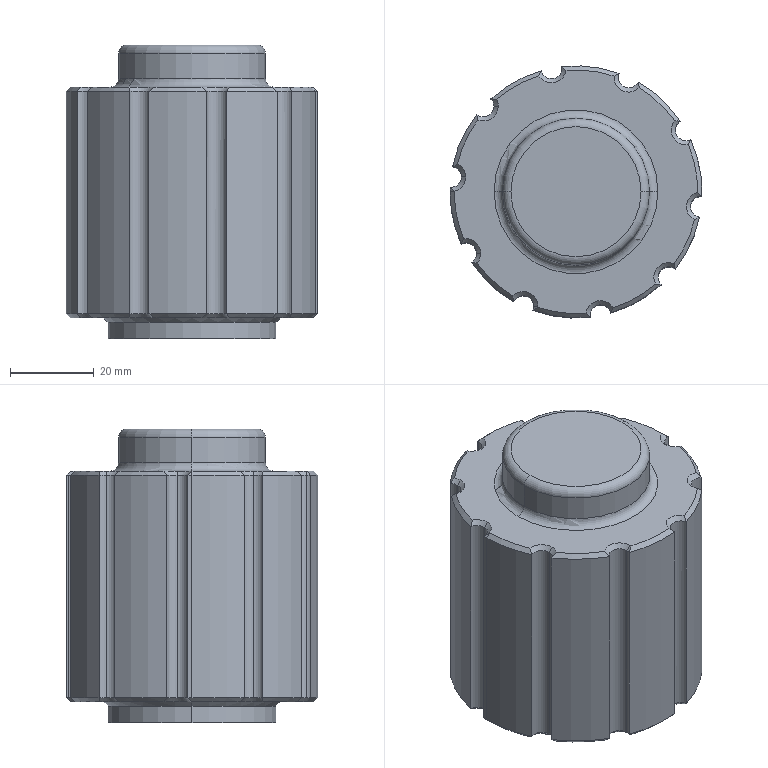Part | SolidWorks | features ICE 2, Chamfer 1, Cut 1, Extrusion 1, Fillet 1 | 1 solid | 92 faces | box 60 x 60 x 70 mm | volume 165967 mm3 | cone 54 | cylinder 30 | torus 4 | plane 4 | commonest cylinder face diameters 5 x15 60 x11 35 x2 40 x2